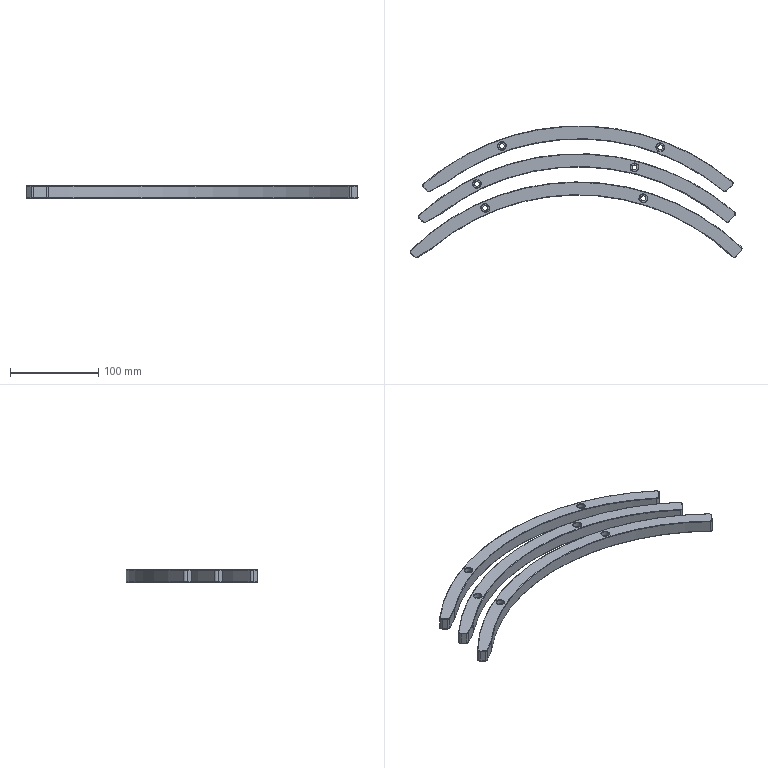Part | 3 solids | 120 faces | box 376.065 x 149.521 x 14 mm | volume 239699 mm3 | cylinder 51 | torus 42 | plane 21 | cone 6 | commonest cylinder face diameters 1 x18 6 x7 5.5 x6 9 x6 4 x5 40 x3